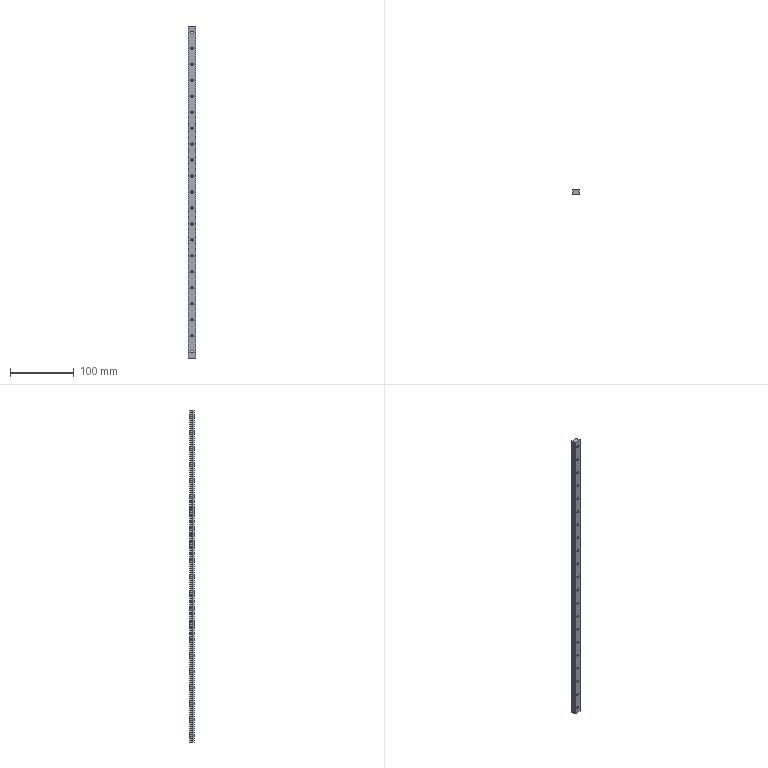Part | NX | features BREP 1 | 1 solid | 123 faces | box 12 x 7.5 x 520 mm | volume 39830 mm3 | cylinder 84 | plane 39 | commonest cylinder face diameters 3.5 x42 6 x42